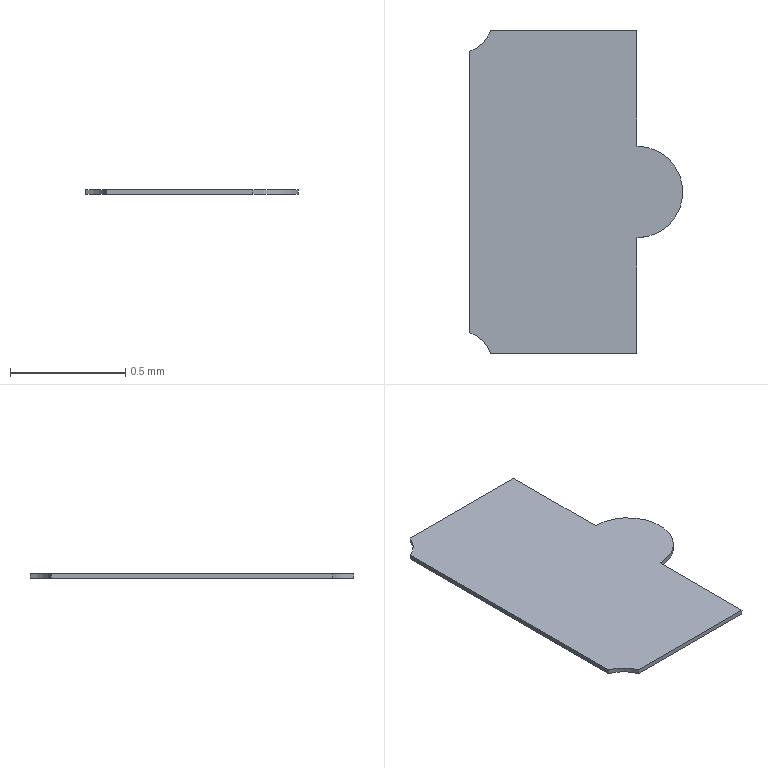Part | STEP file | RJ-USIO-V1_2-220411_27 | 1 solid | 10 faces | box 0.9234 x 1.4 x 0.02 mm | volume 0.02132 mm3 | plane 7 | cylinder 3 | commonest cylinder face diameters 0.3 x2 0.397 x1
STEP:
#1=CARTESIAN_POINT('',(0.,0.,0.));
#2=DIRECTION('',(0.,0.,1.));
#3=DIRECTION('',(1.,0.,0.));
#4=AXIS2_PLACEMENT_3D('',#1,#2,#3);
#5=CARTESIAN_POINT('',(38.925,55.398,0.000000009));
#6=VERTEX_POINT('',#5);
#7=CARTESIAN_POINT('',(38.925,55.001,-0.000000009));
#8=VERTEX_POINT('',#7);
#9=CARTESIAN_POINT('',(38.925,55.2,0.));
#10=DIRECTION('',(0.,0.000000044,-1.));
#11=DIRECTION('',(-0.000000175,1.,0.000000044));
#12=AXIS2_PLACEMENT_3D('',#9,#10,#11);
#13=CIRCLE('',#12,0.1984);
#14=CARTESIAN_POINT('',(38.925,55.2,0.));
#15=DIRECTION('',(0.,0.000000044,-1.));
#16=DIRECTION('',(0.000000175,-1.,-0.000000044));
#17=AXIS2_PLACEMENT_3D('',#14,#15,#16);
#18=PLANE('',#17);
#19=CARTESIAN_POINT('',(0.,0.));
#20=DIRECTION('',(-1.,0.));
#21=AXIS2_PLACEMENT_2D('',#19,#20);
#22=CIRCLE('',#21,0.1984);
#23=(GEOMETRIC_REPRESENTATION_CONTEXT(2)PARAMETRIC_REPRESENTATION_CONTEXT()REPRESENTATION_CONTEXT('',''));
#24=DEFINITIONAL_REPRESENTATION('',(#22),#23);
#25=PCURVE('',#18,#24);
#26=CARTESIAN_POINT('',(38.925,55.2,0.02));
#27=DIRECTION('',(0.,0.000000044,-1.));
#28=DIRECTION('',(0.000000175,-1.,-0.000000044));
#29=AXIS2_PLACEMENT_3D('',#26,#27,#28);
#30=CYLINDRICAL_SURFACE('',#29,0.1984);
#31=CARTESIAN_POINT('',(3.142,0.02));
#32=DIRECTION('',(1.,0.));
#33=VECTOR('',#32,1.);
#34=LINE('',#31,#33);
#35=(GEOMETRIC_REPRESENTATION_CONTEXT(2)PARAMETRIC_REPRESENTATION_CONTEXT()REPRESENTATION_CONTEXT('',''));
#36=DEFINITIONAL_REPRESENTATION('',(#34),#35);
#37=PCURVE('',#30,#36);
#38=SURFACE_CURVE('',#13,(#25,#37),.PCURVE_S1.);
#39=EDGE_CURVE('',#6,#8,#38,.T.);
#40=ORIENTED_EDGE('',*,*,#39,.F.);
#41=CARTESIAN_POINT('',(38.925,55.9,0.000000031));
#42=VERTEX_POINT('',#41);
#43=CARTESIAN_POINT('',(38.925,55.9,0.000000031));
#44=DIRECTION('',(0.000000175,-1.,-0.000000044));
#45=VECTOR('',#44,1.);
#46=LINE('',#43,#45);
#47=CARTESIAN_POINT('',(-0.7,0.));
#48=DIRECTION('',(1.,0.));
#49=VECTOR('',#48,1.);
#50=LINE('',#47,#49);
#51=(GEOMETRIC_REPRESENTATION_CONTEXT(2)PARAMETRIC_REPRESENTATION_CONTEXT()REPRESENTATION_CONTEXT('',''));
#52=DEFINITIONAL_REPRESENTATION('',(#50),#51);
#53=PCURVE('',#18,#52);
#54=CARTESIAN_POINT('',(38.925,55.9,0.02));
#55=DIRECTION('',(-1.,-0.000000175,0.));
#56=DIRECTION('',(-0.000000175,1.,0.000000044));
#57=AXIS2_PLACEMENT_3D('',#54,#55,#56);
#58=PLANE('',#57);
#59=CARTESIAN_POINT('',(0.,0.02));
#60=DIRECTION('',(-1.,0.));
#61=VECTOR('',#60,1.);
#62=LINE('',#59,#61);
#63=(GEOMETRIC_REPRESENTATION_CONTEXT(2)PARAMETRIC_REPRESENTATION_CONTEXT()REPRESENTATION_CONTEXT('',''));
#64=DEFINITIONAL_REPRESENTATION('',(#62),#63);
#65=PCURVE('',#58,#64);
#66=SURFACE_CURVE('',#46,(#53,#65),.PCURVE_S1.);
#67=EDGE_CURVE('',#42,#6,#66,.T.);
#68=ORIENTED_EDGE('',*,*,#67,.F.);
#69=CARTESIAN_POINT('',(38.291,55.9,0.000000031));
#70=VERTEX_POINT('',#69);
#71=CARTESIAN_POINT('',(38.291,55.9,0.000000031));
#72=DIRECTION('',(1.,0.000000175,0.));
#73=VECTOR('',#72,1.);
#74=LINE('',#71,#73);
#75=CARTESIAN_POINT('',(-0.7,0.6336));
#76=DIRECTION('',(0.,-1.));
#77=VECTOR('',#76,1.);
#78=LINE('',#75,#77);
#79=(GEOMETRIC_REPRESENTATION_CONTEXT(2)PARAMETRIC_REPRESENTATION_CONTEXT()REPRESENTATION_CONTEXT('',''));
#80=DEFINITIONAL_REPRESENTATION('',(#78),#79);
#81=PCURVE('',#18,#80);
#82=CARTESIAN_POINT('',(38.291,55.9,0.02));
#83=DIRECTION('',(0.000000175,-1.,-0.000000044));
#84=DIRECTION('',(-1.,-0.000000175,0.));
#85=AXIS2_PLACEMENT_3D('',#82,#83,#84);
#86=PLANE('',#85);
#87=CARTESIAN_POINT('',(0.,0.02));
#88=DIRECTION('',(-1.,0.));
#89=VECTOR('',#88,1.);
#90=LINE('',#87,#89);
#91=(GEOMETRIC_REPRESENTATION_CONTEXT(2)PARAMETRIC_REPRESENTATION_CONTEXT()REPRESENTATION_CONTEXT('',''));
#92=DEFINITIONAL_REPRESENTATION('',(#90),#91);
#93=PCURVE('',#86,#92);
#94=SURFACE_CURVE('',#74,(#81,#93),.PCURVE_S1.);
#95=EDGE_CURVE('',#70,#42,#94,.T.);
#96=ORIENTED_EDGE('',*,*,#95,.F.);
#97=CARTESIAN_POINT('',(38.2,55.808,0.000000027));
#98=VERTEX_POINT('',#97);
#99=CARTESIAN_POINT('',(38.15,55.95,0.000000033));
#100=DIRECTION('',(0.,-0.000000044,1.));
#101=DIRECTION('',(0.3333,-0.9428,-0.000000041));
#102=AXIS2_PLACEMENT_3D('',#99,#100,#101);
#103=CIRCLE('',#102,0.15);
#104=CARTESIAN_POINT('',(-0.6086,0.725));
#105=CARTESIAN_POINT('',(-0.6952,0.4801));
#106=CARTESIAN_POINT('',(-0.864,0.6775));
#107=CARTESIAN_POINT('',(-1.033,0.875));
#108=CARTESIAN_POINT('',(-0.7774,0.9225));
#109=CARTESIAN_POINT('',(-0.522,0.9699));
#110=CARTESIAN_POINT('',(-0.6086,0.725));
#111=(BOUNDED_CURVE()B_SPLINE_CURVE(2,(#104,#105,#106,#107,#108,#109,#110),.UNSPECIFIED.,.T.,.F.)B_SPLINE_CURVE_WITH_KNOTS((1,2,2,2,2,1),(-2.094,0.,2.094,4.189,6.283,8.378),.UNSPECIFIED.)CURVE()GEOMETRIC_REPRESENTATION_ITEM()RATIONAL_B_SPLINE_CURVE((1.,0.5,1.,0.5,1.,0.5,1.))REPRESENTATION_ITEM(''));
#112=(GEOMETRIC_REPRESENTATION_CONTEXT(2)PARAMETRIC_REPRESENTATION_CONTEXT()REPRESENTATION_CONTEXT('',''));
#113=DEFINITIONAL_REPRESENTATION('',(#111),#112);
#114=PCURVE('',#18,#113);
#115=CARTESIAN_POINT('',(38.15,55.95,0.02));
#116=DIRECTION('',(0.,0.000000044,-1.));
#117=DIRECTION('',(0.000000175,-1.,-0.000000044));
#118=AXIS2_PLACEMENT_3D('',#115,#116,#117);
#119=CYLINDRICAL_SURFACE('',#118,0.15);
#120=CARTESIAN_POINT('',(5.943,0.02));
#121=DIRECTION('',(-1.,0.));
#122=VECTOR('',#121,1.);
#123=LINE('',#120,#122);
#124=(GEOMETRIC_REPRESENTATION_CONTEXT(2)PARAMETRIC_REPRESENTATION_CONTEXT()REPRESENTATION_CONTEXT('',''));
#125=DEFINITIONAL_REPRESENTATION('',(#123),#124);
#126=PCURVE('',#119,#125);
#127=SURFACE_CURVE('',#103,(#114,#126),.PCURVE_S1.);
#128=EDGE_CURVE('',#98,#70,#127,.T.);
#129=ORIENTED_EDGE('',*,*,#128,.F.);
#130=CARTESIAN_POINT('',(38.2,54.591,-0.000000027));
#131=VERTEX_POINT('',#130);
#132=CARTESIAN_POINT('',(38.2,54.591,-0.000000027));
#133=DIRECTION('',(-0.000000175,1.,0.000000044));
#134=VECTOR('',#133,1.);
#135=LINE('',#132,#134);
#136=CARTESIAN_POINT('',(0.6086,0.725));
#137=DIRECTION('',(-1.,0.));
#138=VECTOR('',#137,1.);
#139=LINE('',#136,#138);
#140=(GEOMETRIC_REPRESENTATION_CONTEXT(2)PARAMETRIC_REPRESENTATION_CONTEXT()REPRESENTATION_CONTEXT('',''));
#141=DEFINITIONAL_REPRESENTATION('',(#139),#140);
#142=PCURVE('',#18,#141);
#143=CARTESIAN_POINT('',(38.2,55.808,0.02));
#144=DIRECTION('',(1.,0.000000175,0.));
#145=DIRECTION('',(0.000000175,-1.,-0.000000044));
#146=AXIS2_PLACEMENT_3D('',#143,#144,#145);
#147=PLANE('',#146);
#148=CARTESIAN_POINT('',(1.217,0.02));
#149=DIRECTION('',(-1.,0.));
#150=VECTOR('',#149,1.);
#151=LINE('',#148,#150);
#152=(GEOMETRIC_REPRESENTATION_CONTEXT(2)PARAMETRIC_REPRESENTATION_CONTEXT()REPRESENTATION_CONTEXT('',''));
#153=DEFINITIONAL_REPRESENTATION('',(#151),#152);
#154=PCURVE('',#147,#153);
#155=SURFACE_CURVE('',#135,(#142,#154),.PCURVE_S1.);
#156=EDGE_CURVE('',#131,#98,#155,.T.);
#157=ORIENTED_EDGE('',*,*,#156,.F.);
#158=CARTESIAN_POINT('',(38.291,54.5,-0.000000031));
#159=VERTEX_POINT('',#158);
#160=CARTESIAN_POINT('',(38.15,54.45,-0.000000033));
#161=DIRECTION('',(0.,-0.000000044,1.));
#162=DIRECTION('',(0.9428,0.3333,0.000000015));
#163=AXIS2_PLACEMENT_3D('',#160,#161,#162);
#164=CIRCLE('',#163,0.15);
#165=CARTESIAN_POINT('',(0.7,0.6336));
#166=CARTESIAN_POINT('',(0.4551,0.7202));
#167=CARTESIAN_POINT('',(0.6525,0.889));
#168=CARTESIAN_POINT('',(0.85,1.058));
#169=CARTESIAN_POINT('',(0.8975,0.8024));
#170=CARTESIAN_POINT('',(0.9449,0.547));
#171=CARTESIAN_POINT('',(0.7,0.6336));
#172=(BOUNDED_CURVE()B_SPLINE_CURVE(2,(#165,#166,#167,#168,#169,#170,#171),.UNSPECIFIED.,.T.,.F.)B_SPLINE_CURVE_WITH_KNOTS((1,2,2,2,2,1),(-2.094,0.,2.094,4.189,6.283,8.378),.UNSPECIFIED.)CURVE()GEOMETRIC_REPRESENTATION_ITEM()RATIONAL_B_SPLINE_CURVE((1.,0.5,1.,0.5,1.,0.5,1.))REPRESENTATION_ITEM(''));
#173=(GEOMETRIC_REPRESENTATION_CONTEXT(2)PARAMETRIC_REPRESENTATION_CONTEXT()REPRESENTATION_CONTEXT('',''));
#174=DEFINITIONAL_REPRESENTATION('',(#172),#173);
#175=PCURVE('',#18,#174);
#176=CARTESIAN_POINT('',(38.15,54.45,0.02));
#177=DIRECTION('',(0.,0.000000044,-1.));
#178=DIRECTION('',(0.000000175,-1.,-0.000000044));
#179=AXIS2_PLACEMENT_3D('',#176,#177,#178);
#180=CYLINDRICAL_SURFACE('',#179,0.15);
#181=CARTESIAN_POINT('',(4.373,0.02));
#182=DIRECTION('',(-1.,0.));
#183=VECTOR('',#182,1.);
#184=LINE('',#181,#183);
#185=(GEOMETRIC_REPRESENTATION_CONTEXT(2)PARAMETRIC_REPRESENTATION_CONTEXT()REPRESENTATION_CONTEXT('',''));
#186=DEFINITIONAL_REPRESENTATION('',(#184),#185);
#187=PCURVE('',#180,#186);
#188=SURFACE_CURVE('',#164,(#175,#187),.PCURVE_S1.);
#189=EDGE_CURVE('',#159,#131,#188,.T.);
#190=ORIENTED_EDGE('',*,*,#189,.F.);
#191=CARTESIAN_POINT('',(38.925,54.5,-0.000000031));
#192=VERTEX_POINT('',#191);
#193=CARTESIAN_POINT('',(38.925,54.5,-0.000000031));
#194=DIRECTION('',(-1.,-0.000000175,0.));
#195=VECTOR('',#194,1.);
#196=LINE('',#193,#195);
#197=CARTESIAN_POINT('',(0.7,0.));
#198=DIRECTION('',(0.,1.));
#199=VECTOR('',#198,1.);
#200=LINE('',#197,#199);
#201=(GEOMETRIC_REPRESENTATION_CONTEXT(2)PARAMETRIC_REPRESENTATION_CONTEXT()REPRESENTATION_CONTEXT('',''));
#202=DEFINITIONAL_REPRESENTATION('',(#200),#201);
#203=PCURVE('',#18,#202);
#204=CARTESIAN_POINT('',(38.925,54.5,0.02));
#205=DIRECTION('',(-0.000000175,1.,0.000000044));
#206=DIRECTION('',(1.,0.000000175,0.));
#207=AXIS2_PLACEMENT_3D('',#204,#205,#206);
#208=PLANE('',#207);
#209=CARTESIAN_POINT('',(0.,0.02));
#210=DIRECTION('',(-1.,0.));
#211=VECTOR('',#210,1.);
#212=LINE('',#209,#211);
#213=(GEOMETRIC_REPRESENTATION_CONTEXT(2)PARAMETRIC_REPRESENTATION_CONTEXT()REPRESENTATION_CONTEXT('',''));
#214=DEFINITIONAL_REPRESENTATION('',(#212),#213);
#215=PCURVE('',#208,#214);
#216=SURFACE_CURVE('',#196,(#203,#215),.PCURVE_S1.);
#217=EDGE_CURVE('',#192,#159,#216,.T.);
#218=ORIENTED_EDGE('',*,*,#217,.F.);
#219=CARTESIAN_POINT('',(38.925,55.001,-0.000000009));
#220=DIRECTION('',(0.000000175,-1.,-0.000000044));
#221=VECTOR('',#220,1.);
#222=LINE('',#219,#221);
#223=CARTESIAN_POINT('',(0.1984,0.));
#224=DIRECTION('',(1.,0.));
#225=VECTOR('',#224,1.);
#226=LINE('',#223,#225);
#227=(GEOMETRIC_REPRESENTATION_CONTEXT(2)PARAMETRIC_REPRESENTATION_CONTEXT()REPRESENTATION_CONTEXT('',''));
#228=DEFINITIONAL_REPRESENTATION('',(#226),#227);
#229=PCURVE('',#18,#228);
#230=CARTESIAN_POINT('',(38.925,55.001,0.02));
#231=DIRECTION('',(-1.,-0.000000175,0.));
#232=DIRECTION('',(-0.000000175,1.,0.000000044));
#233=AXIS2_PLACEMENT_3D('',#230,#231,#232);
#234=PLANE('',#233);
#235=CARTESIAN_POINT('',(0.,0.02));
#236=DIRECTION('',(-1.,0.));
#237=VECTOR('',#236,1.);
#238=LINE('',#235,#237);
#239=(GEOMETRIC_REPRESENTATION_CONTEXT(2)PARAMETRIC_REPRESENTATION_CONTEXT()REPRESENTATION_CONTEXT('',''));
#240=DEFINITIONAL_REPRESENTATION('',(#238),#239);
#241=PCURVE('',#234,#240);
#242=SURFACE_CURVE('',#222,(#229,#241),.PCURVE_S1.);
#243=EDGE_CURVE('',#8,#192,#242,.T.);
#244=ORIENTED_EDGE('',*,*,#243,.F.);
#245=EDGE_LOOP('',(#40,#68,#96,#129,#157,#190,#218,#244));
#246=FACE_BOUND('',#245,.F.);
#247=ADVANCED_FACE('',(#246),#18,.T.);
#248=CARTESIAN_POINT('',(38.925,55.398,0.02));
#249=VERTEX_POINT('',#248);
#250=CARTESIAN_POINT('',(38.925,55.398,0.000000009));
#251=DIRECTION('',(0.,-0.000000044,1.));
#252=VECTOR('',#251,1.);
#253=LINE('',#250,#252);
#254=CARTESIAN_POINT('',(3.142,0.02));
#255=DIRECTION('',(0.,-1.));
#256=VECTOR('',#255,1.);
#257=LINE('',#254,#256);
#258=(GEOMETRIC_REPRESENTATION_CONTEXT(2)PARAMETRIC_REPRESENTATION_CONTEXT()REPRESENTATION_CONTEXT('',''));
#259=DEFINITIONAL_REPRESENTATION('',(#257),#258);
#260=PCURVE('',#30,#259);
#261=CARTESIAN_POINT('',(-0.5016,0.02));
#262=DIRECTION('',(0.,-1.));
#263=VECTOR('',#262,1.);
#264=LINE('',#261,#263);
#265=(GEOMETRIC_REPRESENTATION_CONTEXT(2)PARAMETRIC_REPRESENTATION_CONTEXT()REPRESENTATION_CONTEXT('',''));
#266=DEFINITIONAL_REPRESENTATION('',(#264),#265);
#267=PCURVE('',#58,#266);
#268=SURFACE_CURVE('',#253,(#260,#267),.PCURVE_S1.);
#269=EDGE_CURVE('',#6,#249,#268,.T.);
#270=ORIENTED_EDGE('',*,*,#269,.T.);
#271=CARTESIAN_POINT('',(38.925,55.001,0.02));
#272=VERTEX_POINT('',#271);
#273=CARTESIAN_POINT('',(38.925,55.2,0.02));
#274=DIRECTION('',(0.,-0.000000044,1.));
#275=DIRECTION('',(0.000000175,-1.,-0.000000044));
#276=AXIS2_PLACEMENT_3D('',#273,#274,#275);
#277=CIRCLE('',#276,0.1984);
#278=CARTESIAN_POINT('',(6.283,0.));
#279=DIRECTION('',(-1.,0.));
#280=VECTOR('',#279,1.);
#281=LINE('',#278,#280);
#282=(GEOMETRIC_REPRESENTATION_CONTEXT(2)PARAMETRIC_REPRESENTATION_CONTEXT()REPRESENTATION_CONTEXT('',''));
#283=DEFINITIONAL_REPRESENTATION('',(#281),#282);
#284=PCURVE('',#30,#283);
#285=CARTESIAN_POINT('',(38.925,55.2,0.02));
#286=DIRECTION('',(0.,0.000000044,-1.));
#287=DIRECTION('',(0.000000175,-1.,-0.000000044));
#288=AXIS2_PLACEMENT_3D('',#285,#286,#287);
#289=PLANE('',#288);
#290=CARTESIAN_POINT('',(0.1984,0.));
#291=CARTESIAN_POINT('',(0.1984,-0.3436));
#292=CARTESIAN_POINT('',(-0.09918,-0.1718));
#293=CARTESIAN_POINT('',(-0.3967,0.));
#294=CARTESIAN_POINT('',(-0.09918,0.1718));
#295=CARTESIAN_POINT('',(0.1984,0.3436));
#296=CARTESIAN_POINT('',(0.1984,0.));
#297=(BOUNDED_CURVE()B_SPLINE_CURVE(2,(#290,#291,#292,#293,#294,#295,#296),.UNSPECIFIED.,.T.,.F.)B_SPLINE_CURVE_WITH_KNOTS((1,2,2,2,2,1),(-2.094,0.,2.094,4.189,6.283,8.378),.UNSPECIFIED.)CURVE()GEOMETRIC_REPRESENTATION_ITEM()RATIONAL_B_SPLINE_CURVE((1.,0.5,1.,0.5,1.,0.5,1.))REPRESENTATION_ITEM(''));
#298=(GEOMETRIC_REPRESENTATION_CONTEXT(2)PARAMETRIC_REPRESENTATION_CONTEXT()REPRESENTATION_CONTEXT('',''));
#299=DEFINITIONAL_REPRESENTATION('',(#297),#298);
#300=PCURVE('',#289,#299);
#301=SURFACE_CURVE('',#277,(#284,#300),.PCURVE_S1.);
#302=EDGE_CURVE('',#272,#249,#301,.T.);
#303=ORIENTED_EDGE('',*,*,#302,.F.);
#304=CARTESIAN_POINT('',(38.925,55.001,0.02));
#305=DIRECTION('',(0.,0.000000044,-1.));
#306=VECTOR('',#305,1.);
#307=LINE('',#304,#306);
#308=CARTESIAN_POINT('',(6.283,0.));
#309=DIRECTION('',(0.,1.));
#310=VECTOR('',#309,1.);
#311=LINE('',#308,#310);
#312=(GEOMETRIC_REPRESENTATION_CONTEXT(2)PARAMETRIC_REPRESENTATION_CONTEXT()REPRESENTATION_CONTEXT('',''));
#313=DEFINITIONAL_REPRESENTATION('',(#311),#312);
#314=PCURVE('',#30,#313);
#315=CARTESIAN_POINT('',(0.,0.));
#316=DIRECTION('',(0.,1.));
#317=VECTOR('',#316,1.);
#318=LINE('',#315,#317);
#319=(GEOMETRIC_REPRESENTATION_CONTEXT(2)PARAMETRIC_REPRESENTATION_CONTEXT()REPRESENTATION_CONTEXT('',''));
#320=DEFINITIONAL_REPRESENTATION('',(#318),#319);
#321=PCURVE('',#234,#320);
#322=SURFACE_CURVE('',#307,(#314,#321),.PCURVE_S1.);
#323=EDGE_CURVE('',#272,#8,#322,.T.);
#324=ORIENTED_EDGE('',*,*,#323,.T.);
#325=ORIENTED_EDGE('',*,*,#39,.F.);
#326=EDGE_LOOP('',(#270,#303,#324,#325));
#327=FACE_BOUND('',#326,.T.);
#328=ADVANCED_FACE('',(#327),#30,.T.);
#329=ORIENTED_EDGE('',*,*,#243,.T.);
#330=CARTESIAN_POINT('',(38.925,54.5,0.02));
#331=VERTEX_POINT('',#330);
#332=CARTESIAN_POINT('',(38.925,54.5,-0.000000031));
#333=DIRECTION('',(0.,-0.000000044,1.));
#334=VECTOR('',#333,1.);
#335=LINE('',#332,#334);
#336=CARTESIAN_POINT('',(-0.5016,0.02));
#337=DIRECTION('',(0.,-1.));
#338=VECTOR('',#337,1.);
#339=LINE('',#336,#338);
#340=(GEOMETRIC_REPRESENTATION_CONTEXT(2)PARAMETRIC_REPRESENTATION_CONTEXT()REPRESENTATION_CONTEXT('',''));
#341=DEFINITIONAL_REPRESENTATION('',(#339),#340);
#342=PCURVE('',#234,#341);
#343=CARTESIAN_POINT('',(0.,0.02));
#344=DIRECTION('',(0.,-1.));
#345=VECTOR('',#344,1.);
#346=LINE('',#343,#345);
#347=(GEOMETRIC_REPRESENTATION_CONTEXT(2)PARAMETRIC_REPRESENTATION_CONTEXT()REPRESENTATION_CONTEXT('',''));
#348=DEFINITIONAL_REPRESENTATION('',(#346),#347);
#349=PCURVE('',#208,#348);
#350=SURFACE_CURVE('',#335,(#342,#349),.PCURVE_S1.);
#351=EDGE_CURVE('',#192,#331,#350,.T.);
#352=ORIENTED_EDGE('',*,*,#351,.T.);
#353=CARTESIAN_POINT('',(38.925,55.001,0.02));
#354=DIRECTION('',(0.000000175,-1.,-0.000000044));
#355=VECTOR('',#354,1.);
#356=LINE('',#353,#355);
#357=CARTESIAN_POINT('',(0.,0.));
#358=DIRECTION('',(-1.,0.));
#359=VECTOR('',#358,1.);
#360=LINE('',#357,#359);
#361=(GEOMETRIC_REPRESENTATION_CONTEXT(2)PARAMETRIC_REPRESENTATION_CONTEXT()REPRESENTATION_CONTEXT('',''));
#362=DEFINITIONAL_REPRESENTATION('',(#360),#361);
#363=PCURVE('',#234,#362);
#364=CARTESIAN_POINT('',(0.1984,0.));
#365=DIRECTION('',(1.,0.));
#366=VECTOR('',#365,1.);
#367=LINE('',#364,#366);
#368=(GEOMETRIC_REPRESENTATION_CONTEXT(2)PARAMETRIC_REPRESENTATION_CONTEXT()REPRESENTATION_CONTEXT('',''));
#369=DEFINITIONAL_REPRESENTATION('',(#367),#368);
#370=PCURVE('',#289,#369);
#371=SURFACE_CURVE('',#356,(#363,#370),.PCURVE_S1.);
#372=EDGE_CURVE('',#272,#331,#371,.T.);
#373=ORIENTED_EDGE('',*,*,#372,.F.);
#374=ORIENTED_EDGE('',*,*,#323,.T.);
#375=EDGE_LOOP('',(#329,#352,#373,#374));
#376=FACE_BOUND('',#375,.F.);
#377=ADVANCED_FACE('',(#376),#234,.F.);
#378=ORIENTED_EDGE('',*,*,#217,.T.);
#379=CARTESIAN_POINT('',(38.291,54.5,0.02));
#380=VERTEX_POINT('',#379);
#381=CARTESIAN_POINT('',(38.291,54.5,-0.000000031));
#382=DIRECTION('',(0.,-0.000000044,1.));
#383=VECTOR('',#382,1.);
#384=LINE('',#381,#383);
#385=CARTESIAN_POINT('',(-0.6336,0.02));
#386=DIRECTION('',(0.,-1.));
#387=VECTOR('',#386,1.);
#388=LINE('',#385,#387);
#389=(GEOMETRIC_REPRESENTATION_CONTEXT(2)PARAMETRIC_REPRESENTATION_CONTEXT()REPRESENTATION_CONTEXT('',''));
#390=DEFINITIONAL_REPRESENTATION('',(#388),#389);
#391=PCURVE('',#208,#390);
#392=CARTESIAN_POINT('',(4.373,0.02));
#393=DIRECTION('',(0.,-1.));
#394=VECTOR('',#393,1.);
#395=LINE('',#392,#394);
#396=(GEOMETRIC_REPRESENTATION_CONTEXT(2)PARAMETRIC_REPRESENTATION_CONTEXT()REPRESENTATION_CONTEXT('',''));
#397=DEFINITIONAL_REPRESENTATION('',(#395),#396);
#398=PCURVE('',#180,#397);
#399=SURFACE_CURVE('',#384,(#391,#398),.PCURVE_S1.);
#400=EDGE_CURVE('',#159,#380,#399,.T.);
#401=ORIENTED_EDGE('',*,*,#400,.T.);
#402=CARTESIAN_POINT('',(38.925,54.5,0.02));
#403=DIRECTION('',(-1.,-0.000000175,0.));
#404=VECTOR('',#403,1.);
#405=LINE('',#402,#404);
#406=CARTESIAN_POINT('',(0.,0.));
#407=DIRECTION('',(-1.,0.));
#408=VECTOR('',#407,1.);
#409=LINE('',#406,#408);
#410=(GEOMETRIC_REPRESENTATION_CONTEXT(2)PARAMETRIC_REPRESENTATION_CONTEXT()REPRESENTATION_CONTEXT('',''));
#411=DEFINITIONAL_REPRESENTATION('',(#409),#410);
#412=PCURVE('',#208,#411);
#413=CARTESIAN_POINT('',(0.7,0.));
#414=DIRECTION('',(0.,1.));
#415=VECTOR('',#414,1.);
#416=LINE('',#413,#415);
#417=(GEOMETRIC_REPRESENTATION_CONTEXT(2)PARAMETRIC_REPRESENTATION_CONTEXT()REPRESENTATION_CONTEXT('',''));
#418=DEFINITIONAL_REPRESENTATION('',(#416),#417);
#419=PCURVE('',#289,#418);
#420=SURFACE_CURVE('',#405,(#412,#419),.PCURVE_S1.);
#421=EDGE_CURVE('',#331,#380,#420,.T.);
#422=ORIENTED_EDGE('',*,*,#421,.F.);
#423=ORIENTED_EDGE('',*,*,#351,.F.);
#424=EDGE_LOOP('',(#378,#401,#422,#423));
#425=FACE_BOUND('',#424,.F.);
#426=ADVANCED_FACE('',(#425),#208,.F.);
#427=ORIENTED_EDGE('',*,*,#189,.T.);
#428=CARTESIAN_POINT('',(38.2,54.591,0.02));
#429=VERTEX_POINT('',#428);
#430=CARTESIAN_POINT('',(38.2,54.591,0.02));
#431=DIRECTION('',(0.,0.000000044,-1.));
#432=VECTOR('',#431,1.);
#433=LINE('',#430,#432);
#434=CARTESIAN_POINT('',(3.481,0.));
#435=DIRECTION('',(0.,1.));
#436=VECTOR('',#435,1.);
#437=LINE('',#434,#436);
#438=(GEOMETRIC_REPRESENTATION_CONTEXT(2)PARAMETRIC_REPRESENTATION_CONTEXT()REPRESENTATION_CONTEXT('',''));
#439=DEFINITIONAL_REPRESENTATION('',(#437),#438);
#440=PCURVE('',#180,#439);
#441=CARTESIAN_POINT('',(1.217,0.));
#442=DIRECTION('',(0.,1.));
#443=VECTOR('',#442,1.);
#444=LINE('',#441,#443);
#445=(GEOMETRIC_REPRESENTATION_CONTEXT(2)PARAMETRIC_REPRESENTATION_CONTEXT()REPRESENTATION_CONTEXT('',''));
#446=DEFINITIONAL_REPRESENTATION('',(#444),#445);
#447=PCURVE('',#147,#446);
#448=SURFACE_CURVE('',#433,(#440,#447),.PCURVE_S1.);
#449=EDGE_CURVE('',#429,#131,#448,.T.);
#450=ORIENTED_EDGE('',*,*,#449,.F.);
#451=CARTESIAN_POINT('',(38.15,54.45,0.02));
#452=DIRECTION('',(0.,0.000000044,-1.));
#453=DIRECTION('',(0.3333,0.9428,0.000000041));
#454=AXIS2_PLACEMENT_3D('',#451,#452,#453);
#455=CIRCLE('',#454,0.15);
#456=CARTESIAN_POINT('',(3.481,0.));
#457=DIRECTION('',(1.,0.));
#458=VECTOR('',#457,1.);
#459=LINE('',#456,#458);
#460=(GEOMETRIC_REPRESENTATION_CONTEXT(2)PARAMETRIC_REPRESENTATION_CONTEXT()REPRESENTATION_CONTEXT('',''));
#461=DEFINITIONAL_REPRESENTATION('',(#459),#460);
#462=PCURVE('',#180,#461);
#463=CARTESIAN_POINT('',(0.75,0.775));
#464=DIRECTION('',(-0.9428,-0.3333));
#465=AXIS2_PLACEMENT_2D('',#463,#464);
#466=CIRCLE('',#465,0.15);
#467=(GEOMETRIC_REPRESENTATION_CONTEXT(2)PARAMETRIC_REPRESENTATION_CONTEXT()REPRESENTATION_CONTEXT('',''));
#468=DEFINITIONAL_REPRESENTATION('',(#466),#467);
#469=PCURVE('',#289,#468);
#470=SURFACE_CURVE('',#455,(#462,#469),.PCURVE_S1.);
#471=EDGE_CURVE('',#429,#380,#470,.T.);
#472=ORIENTED_EDGE('',*,*,#471,.T.);
#473=ORIENTED_EDGE('',*,*,#400,.F.);
#474=EDGE_LOOP('',(#427,#450,#472,#473));
#475=FACE_BOUND('',#474,.F.);
#476=ADVANCED_FACE('',(#475),#180,.F.);
#477=ORIENTED_EDGE('',*,*,#156,.T.);
#478=CARTESIAN_POINT('',(38.2,55.808,0.02));
#479=VERTEX_POINT('',#478);
#480=CARTESIAN_POINT('',(38.2,55.808,0.000000027));
#481=DIRECTION('',(0.,-0.000000044,1.));
#482=VECTOR('',#481,1.);
#483=LINE('',#480,#482);
#484=CARTESIAN_POINT('',(0.,0.02));
#485=DIRECTION('',(0.,-1.));
#486=VECTOR('',#485,1.);
#487=LINE('',#484,#486);
#488=(GEOMETRIC_REPRESENTATION_CONTEXT(2)PARAMETRIC_REPRESENTATION_CONTEXT()REPRESENTATION_CONTEXT('',''));
#489=DEFINITIONAL_REPRESENTATION('',(#487),#488);
#490=PCURVE('',#147,#489);
#491=CARTESIAN_POINT('',(5.943,0.02));
#492=DIRECTION('',(0.,-1.));
#493=VECTOR('',#492,1.);
#494=LINE('',#491,#493);
#495=(GEOMETRIC_REPRESENTATION_CONTEXT(2)PARAMETRIC_REPRESENTATION_CONTEXT()REPRESENTATION_CONTEXT('',''));
#496=DEFINITIONAL_REPRESENTATION('',(#494),#495);
#497=PCURVE('',#119,#496);
#498=SURFACE_CURVE('',#483,(#490,#497),.PCURVE_S1.);
#499=EDGE_CURVE('',#98,#479,#498,.T.);
#500=ORIENTED_EDGE('',*,*,#499,.T.);
#501=CARTESIAN_POINT('',(38.2,54.591,0.02));
#502=DIRECTION('',(-0.000000175,1.,0.000000044));
#503=VECTOR('',#502,1.);
#504=LINE('',#501,#503);
#505=CARTESIAN_POINT('',(1.217,0.));
#506=DIRECTION('',(-1.,0.));
#507=VECTOR('',#506,1.);
#508=LINE('',#505,#507);
#509=(GEOMETRIC_REPRESENTATION_CONTEXT(2)PARAMETRIC_REPRESENTATION_CONTEXT()REPRESENTATION_CONTEXT('',''));
#510=DEFINITIONAL_REPRESENTATION('',(#508),#509);
#511=PCURVE('',#147,#510);
#512=CARTESIAN_POINT('',(0.6086,0.725));
#513=DIRECTION('',(-1.,0.));
#514=VECTOR('',#513,1.);
#515=LINE('',#512,#514);
#516=(GEOMETRIC_REPRESENTATION_CONTEXT(2)PARAMETRIC_REPRESENTATION_CONTEXT()REPRESENTATION_CONTEXT('',''));
#517=DEFINITIONAL_REPRESENTATION('',(#515),#516);
#518=PCURVE('',#289,#517);
#519=SURFACE_CURVE('',#504,(#511,#518),.PCURVE_S1.);
#520=EDGE_CURVE('',#429,#479,#519,.T.);
#521=ORIENTED_EDGE('',*,*,#520,.F.);
#522=ORIENTED_EDGE('',*,*,#449,.T.);
#523=EDGE_LOOP('',(#477,#500,#521,#522));
#524=FACE_BOUND('',#523,.F.);
#525=ADVANCED_FACE('',(#524),#147,.F.);
#526=ORIENTED_EDGE('',*,*,#128,.T.);
#527=CARTESIAN_POINT('',(38.291,55.9,0.02));
#528=VERTEX_POINT('',#527);
#529=CARTESIAN_POINT('',(38.291,55.9,0.02));
#530=DIRECTION('',(0.,0.000000044,-1.));
#531=VECTOR('',#530,1.);
#532=LINE('',#529,#531);
#533=CARTESIAN_POINT('',(5.052,0.));
#534=DIRECTION('',(0.,1.));
#535=VECTOR('',#534,1.);
#536=LINE('',#533,#535);
#537=(GEOMETRIC_REPRESENTATION_CONTEXT(2)PARAMETRIC_REPRESENTATION_CONTEXT()REPRESENTATION_CONTEXT('',''));
#538=DEFINITIONAL_REPRESENTATION('',(#536),#537);
#539=PCURVE('',#119,#538);
#540=CARTESIAN_POINT('',(0.,0.));
#541=DIRECTION('',(0.,1.));
#542=VECTOR('',#541,1.);
#543=LINE('',#540,#542);
#544=(GEOMETRIC_REPRESENTATION_CONTEXT(2)PARAMETRIC_REPRESENTATION_CONTEXT()REPRESENTATION_CONTEXT('',''));
#545=DEFINITIONAL_REPRESENTATION('',(#543),#544);
#546=PCURVE('',#86,#545);
#547=SURFACE_CURVE('',#532,(#539,#546),.PCURVE_S1.);
#548=EDGE_CURVE('',#528,#70,#547,.T.);
#549=ORIENTED_EDGE('',*,*,#548,.F.);
#550=CARTESIAN_POINT('',(38.15,55.95,0.02));
#551=DIRECTION('',(0.,0.000000044,-1.));
#552=DIRECTION('',(0.9428,-0.3333,-0.000000015));
#553=AXIS2_PLACEMENT_3D('',#550,#551,#552);
#554=CIRCLE('',#553,0.15);
#555=CARTESIAN_POINT('',(5.052,0.));
#556=DIRECTION('',(1.,0.));
#557=VECTOR('',#556,1.);
#558=LINE('',#555,#557);
#559=(GEOMETRIC_REPRESENTATION_CONTEXT(2)PARAMETRIC_REPRESENTATION_CONTEXT()REPRESENTATION_CONTEXT('',''));
#560=DEFINITIONAL_REPRESENTATION('',(#558),#559);
#561=PCURVE('',#119,#560);
#562=CARTESIAN_POINT('',(-0.75,0.775));
#563=DIRECTION('',(0.3333,-0.9428));
#564=AXIS2_PLACEMENT_2D('',#562,#563);
#565=CIRCLE('',#564,0.15);
#566=(GEOMETRIC_REPRESENTATION_CONTEXT(2)PARAMETRIC_REPRESENTATION_CONTEXT()REPRESENTATION_CONTEXT('',''));
#567=DEFINITIONAL_REPRESENTATION('',(#565),#566);
#568=PCURVE('',#289,#567);
#569=SURFACE_CURVE('',#554,(#561,#568),.PCURVE_S1.);
#570=EDGE_CURVE('',#528,#479,#569,.T.);
#571=ORIENTED_EDGE('',*,*,#570,.T.);
#572=ORIENTED_EDGE('',*,*,#499,.F.);
#573=EDGE_LOOP('',(#526,#549,#571,#572));
#574=FACE_BOUND('',#573,.F.);
#575=ADVANCED_FACE('',(#574),#119,.F.);
#576=ORIENTED_EDGE('',*,*,#95,.T.);
#577=CARTESIAN_POINT('',(38.925,55.9,0.02));
#578=VERTEX_POINT('',#577);
#579=CARTESIAN_POINT('',(38.925,55.9,0.000000031));
#580=DIRECTION('',(0.,-0.000000044,1.));
#581=VECTOR('',#580,1.);
#582=LINE('',#579,#581);
#583=CARTESIAN_POINT('',(-0.6336,0.02));
#584=DIRECTION('',(0.,-1.));
#585=VECTOR('',#584,1.);
#586=LINE('',#583,#585);
#587=(GEOMETRIC_REPRESENTATION_CONTEXT(2)PARAMETRIC_REPRESENTATION_CONTEXT()REPRESENTATION_CONTEXT('',''));
#588=DEFINITIONAL_REPRESENTATION('',(#586),#587);
#589=PCURVE('',#86,#588);
#590=CARTESIAN_POINT('',(0.,0.02));
#591=DIRECTION('',(0.,-1.));
#592=VECTOR('',#591,1.);
#593=LINE('',#590,#592);
#594=(GEOMETRIC_REPRESENTATION_CONTEXT(2)PARAMETRIC_REPRESENTATION_CONTEXT()REPRESENTATION_CONTEXT('',''));
#595=DEFINITIONAL_REPRESENTATION('',(#593),#594);
#596=PCURVE('',#58,#595);
#597=SURFACE_CURVE('',#582,(#589,#596),.PCURVE_S1.);
#598=EDGE_CURVE('',#42,#578,#597,.T.);
#599=ORIENTED_EDGE('',*,*,#598,.T.);
#600=CARTESIAN_POINT('',(38.291,55.9,0.02));
#601=DIRECTION('',(1.,0.000000175,0.));
#602=VECTOR('',#601,1.);
#603=LINE('',#600,#602);
#604=CARTESIAN_POINT('',(0.,0.));
#605=DIRECTION('',(-1.,0.));
#606=VECTOR('',#605,1.);
#607=LINE('',#604,#606);
#608=(GEOMETRIC_REPRESENTATION_CONTEXT(2)PARAMETRIC_REPRESENTATION_CONTEXT()REPRESENTATION_CONTEXT('',''));
#609=DEFINITIONAL_REPRESENTATION('',(#607),#608);
#610=PCURVE('',#86,#609);
#611=CARTESIAN_POINT('',(-0.7,0.6336));
#612=DIRECTION('',(0.,-1.));
#613=VECTOR('',#612,1.);
#614=LINE('',#611,#613);
#615=(GEOMETRIC_REPRESENTATION_CONTEXT(2)PARAMETRIC_REPRESENTATION_CONTEXT()REPRESENTATION_CONTEXT('',''));
#616=DEFINITIONAL_REPRESENTATION('',(#614),#615);
#617=PCURVE('',#289,#616);
#618=SURFACE_CURVE('',#603,(#610,#617),.PCURVE_S1.);
#619=EDGE_CURVE('',#528,#578,#618,.T.);
#620=ORIENTED_EDGE('',*,*,#619,.F.);
#621=ORIENTED_EDGE('',*,*,#548,.T.);
#622=EDGE_LOOP('',(#576,#599,#620,#621));
#623=FACE_BOUND('',#622,.F.);
#624=ADVANCED_FACE('',(#623),#86,.F.);
#625=ORIENTED_EDGE('',*,*,#67,.T.);
#626=ORIENTED_EDGE('',*,*,#269,.T.);
#627=CARTESIAN_POINT('',(38.925,55.9,0.02));
#628=DIRECTION('',(0.000000175,-1.,-0.000000044));
#629=VECTOR('',#628,1.);
#630=LINE('',#627,#629);
#631=CARTESIAN_POINT('',(0.,0.));
#632=DIRECTION('',(-1.,0.));
#633=VECTOR('',#632,1.);
#634=LINE('',#631,#633);
#635=(GEOMETRIC_REPRESENTATION_CONTEXT(2)PARAMETRIC_REPRESENTATION_CONTEXT()REPRESENTATION_CONTEXT('',''));
#636=DEFINITIONAL_REPRESENTATION('',(#634),#635);
#637=PCURVE('',#58,#636);
#638=CARTESIAN_POINT('',(-0.7,0.));
#639=DIRECTION('',(1.,0.));
#640=VECTOR('',#639,1.);
#641=LINE('',#638,#640);
#642=(GEOMETRIC_REPRESENTATION_CONTEXT(2)PARAMETRIC_REPRESENTATION_CONTEXT()REPRESENTATION_CONTEXT('',''));
#643=DEFINITIONAL_REPRESENTATION('',(#641),#642);
#644=PCURVE('',#289,#643);
#645=SURFACE_CURVE('',#630,(#637,#644),.PCURVE_S1.);
#646=EDGE_CURVE('',#578,#249,#645,.T.);
#647=ORIENTED_EDGE('',*,*,#646,.F.);
#648=ORIENTED_EDGE('',*,*,#598,.F.);
#649=EDGE_LOOP('',(#625,#626,#647,#648));
#650=FACE_BOUND('',#649,.F.);
#651=ADVANCED_FACE('',(#650),#58,.F.);
#652=ORIENTED_EDGE('',*,*,#302,.F.);
#653=ORIENTED_EDGE('',*,*,#372,.T.);
#654=ORIENTED_EDGE('',*,*,#421,.T.);
#655=ORIENTED_EDGE('',*,*,#471,.F.);
#656=ORIENTED_EDGE('',*,*,#520,.T.);
#657=ORIENTED_EDGE('',*,*,#570,.F.);
#658=ORIENTED_EDGE('',*,*,#619,.T.);
#659=ORIENTED_EDGE('',*,*,#646,.T.);
#660=EDGE_LOOP('',(#652,#653,#654,#655,#656,#657,#658,#659));
#661=FACE_BOUND('',#660,.F.);
#662=ADVANCED_FACE('',(#661),#289,.F.);
#663=CLOSED_SHELL('',(#247,#328,#377,#426,#476,#525,#575,#624,#651,#662));
#664=MANIFOLD_SOLID_BREP('',#663);
#665=(LENGTH_UNIT()NAMED_UNIT(*)SI_UNIT(.MILLI.,.METRE.));
#666=UNCERTAINTY_MEASURE_WITH_UNIT(LENGTH_MEASURE(0.0000001),#665,'','');
#667=(NAMED_UNIT(*)PLANE_ANGLE_UNIT()SI_UNIT($,.RADIAN.));
#668=(NAMED_UNIT(*)SI_UNIT($,.STERADIAN.)SOLID_ANGLE_UNIT());
#669=(GEOMETRIC_REPRESENTATION_CONTEXT(3)GLOBAL_UNCERTAINTY_ASSIGNED_CONTEXT((#666))GLOBAL_UNIT_ASSIGNED_CONTEXT((#665,#667,#668))REPRESENTATION_CONTEXT('',''));
#670=ADVANCED_BREP_SHAPE_REPRESENTATION('',(#4,#664),#669);